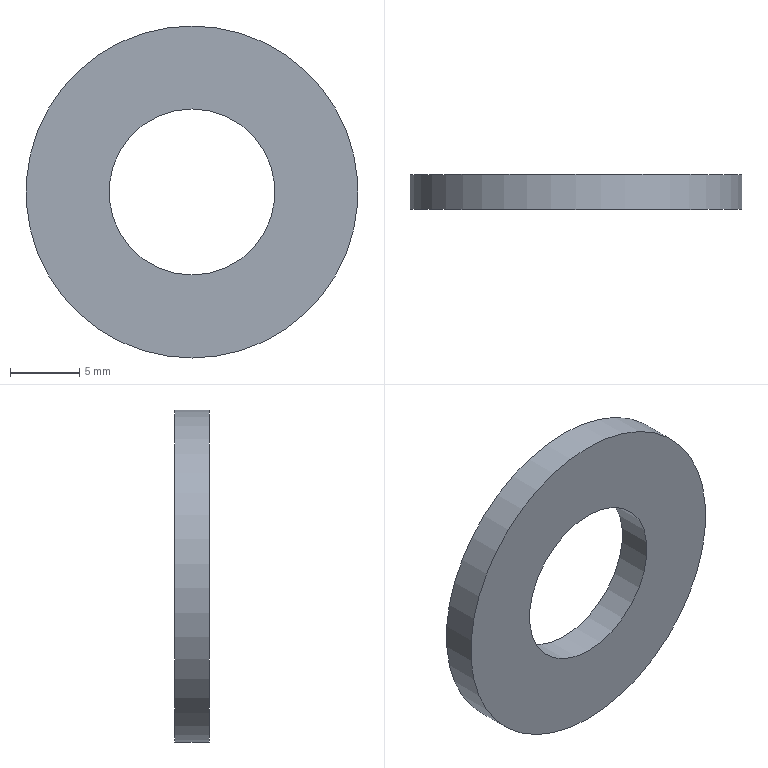Part | NX | features solid 2 | 1 solid | 4 faces | box 24 x 2.5 x 24 mm | volume 848.23 mm3 | plane 2 | cylinder 2 | commonest cylinder face diameters 12 x1 24 x1
STEP:
#1=CARTESIAN_POINT('',(460.,468.,-19.));
#2=VERTEX_POINT('',#1);
#3=CARTESIAN_POINT('',(460.,468.,-25.));
#4=DIRECTION('',(0.,1.,0.));
#5=DIRECTION('',(0.,0.,1.));
#6=AXIS2_PLACEMENT_3D('',#3,#4,#5);
#7=CIRCLE('',#6,6.);
#8=EDGE_CURVE('',#2,#2,#7,.F.);
#9=ORIENTED_EDGE('',*,*,#8,.F.);
#10=EDGE_LOOP('',(#9));
#11=FACE_BOUND('',#10,.T.);
#12=CARTESIAN_POINT('',(460.,468.,-37.));
#13=VERTEX_POINT('',#12);
#14=CARTESIAN_POINT('',(460.,468.,-25.));
#15=DIRECTION('',(0.,-1.,0.));
#16=DIRECTION('',(0.,0.,-1.));
#17=AXIS2_PLACEMENT_3D('',#14,#15,#16);
#18=CIRCLE('',#17,12.);
#19=EDGE_CURVE('',#13,#13,#18,.T.);
#20=ORIENTED_EDGE('',*,*,#19,.T.);
#21=EDGE_LOOP('',(#20));
#22=FACE_BOUND('',#21,.T.);
#23=CARTESIAN_POINT('',(460.,468.,-25.));
#24=DIRECTION('',(0.,-1.,0.));
#25=DIRECTION('',(0.,0.,1.));
#26=AXIS2_PLACEMENT_3D('',#23,#24,#25);
#27=PLANE('',#26);
#28=ADVANCED_FACE('',(#11,#22),#27,.T.);
#29=CARTESIAN_POINT('',(460.,470.5,-19.));
#30=VERTEX_POINT('',#29);
#31=CARTESIAN_POINT('',(460.,470.5,-25.));
#32=DIRECTION('',(0.,1.,0.));
#33=DIRECTION('',(0.,0.,1.));
#34=AXIS2_PLACEMENT_3D('',#31,#32,#33);
#35=CIRCLE('',#34,6.);
#36=EDGE_CURVE('',#30,#30,#35,.F.);
#37=ORIENTED_EDGE('',*,*,#36,.T.);
#38=EDGE_LOOP('',(#37));
#39=FACE_BOUND('',#38,.T.);
#40=CARTESIAN_POINT('',(460.,470.5,-37.));
#41=VERTEX_POINT('',#40);
#42=CARTESIAN_POINT('',(460.,470.5,-25.));
#43=DIRECTION('',(0.,-1.,0.));
#44=DIRECTION('',(0.,0.,-1.));
#45=AXIS2_PLACEMENT_3D('',#42,#43,#44);
#46=CIRCLE('',#45,12.);
#47=EDGE_CURVE('',#41,#41,#46,.T.);
#48=ORIENTED_EDGE('',*,*,#47,.F.);
#49=EDGE_LOOP('',(#48));
#50=FACE_BOUND('',#49,.T.);
#51=CARTESIAN_POINT('',(460.,470.5,-25.));
#52=DIRECTION('',(0.,-1.,0.));
#53=DIRECTION('',(0.,0.,1.));
#54=AXIS2_PLACEMENT_3D('',#51,#52,#53);
#55=PLANE('',#54);
#56=ADVANCED_FACE('',(#39,#50),#55,.F.);
#57=ORIENTED_EDGE('',*,*,#8,.T.);
#58=EDGE_LOOP('',(#57));
#59=FACE_BOUND('',#58,.T.);
#60=ORIENTED_EDGE('',*,*,#36,.F.);
#61=EDGE_LOOP('',(#60));
#62=FACE_BOUND('',#61,.T.);
#63=CARTESIAN_POINT('',(460.,470.5,-25.));
#64=DIRECTION('',(0.,-1.,0.));
#65=DIRECTION('',(0.,0.,1.));
#66=AXIS2_PLACEMENT_3D('',#63,#64,#65);
#67=CYLINDRICAL_SURFACE('',#66,6.);
#68=ADVANCED_FACE('',(#59,#62),#67,.F.);
#69=ORIENTED_EDGE('',*,*,#19,.F.);
#70=EDGE_LOOP('',(#69));
#71=FACE_BOUND('',#70,.T.);
#72=ORIENTED_EDGE('',*,*,#47,.T.);
#73=EDGE_LOOP('',(#72));
#74=FACE_BOUND('',#73,.T.);
#75=CARTESIAN_POINT('',(460.,470.5,-25.));
#76=DIRECTION('',(0.,-1.,0.));
#77=DIRECTION('',(0.,0.,1.));
#78=AXIS2_PLACEMENT_3D('',#75,#76,#77);
#79=CYLINDRICAL_SURFACE('',#78,12.);
#80=ADVANCED_FACE('',(#71,#74),#79,.T.);
#81=CLOSED_SHELL('',(#28,#56,#68,#80));
#82=MANIFOLD_SOLID_BREP('',#81);
#83=(LENGTH_UNIT()NAMED_UNIT(*)SI_UNIT(.MILLI.,.METRE.));
#84=UNCERTAINTY_MEASURE_WITH_UNIT(LENGTH_MEASURE(0.00001),#83,'','');
#85=(NAMED_UNIT(*)PLANE_ANGLE_UNIT()SI_UNIT($,.RADIAN.));
#86=(NAMED_UNIT(*)SI_UNIT($,.STERADIAN.)SOLID_ANGLE_UNIT());
#87=(GEOMETRIC_REPRESENTATION_CONTEXT(3)GLOBAL_UNCERTAINTY_ASSIGNED_CONTEXT((#84))GLOBAL_UNIT_ASSIGNED_CONTEXT((#83,#85,#86))REPRESENTATION_CONTEXT('',''));
#88=ADVANCED_BREP_SHAPE_REPRESENTATION('',(#82),#87);